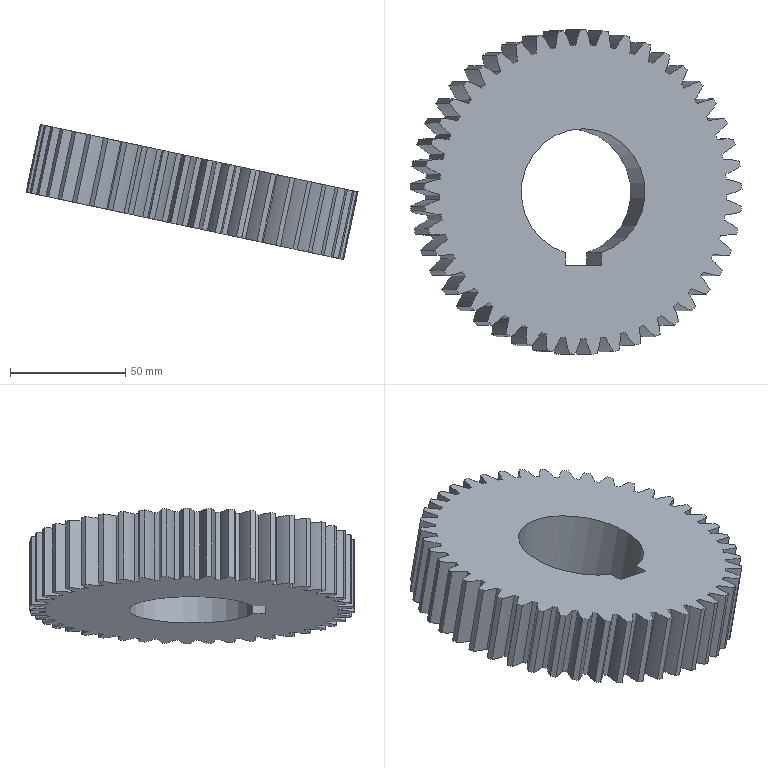Part | STEP file | HL4GZ-1.862.552 (cutter mechanism large gear) | 1 solid | 186 faces | box 144.135 x 140.903 x 58.656 mm | volume 353451 mm3 | cylinder 181 | plane 5 | commonest cylinder face diameters 69.647 x90 127.5 x45 141 x45 55 x1